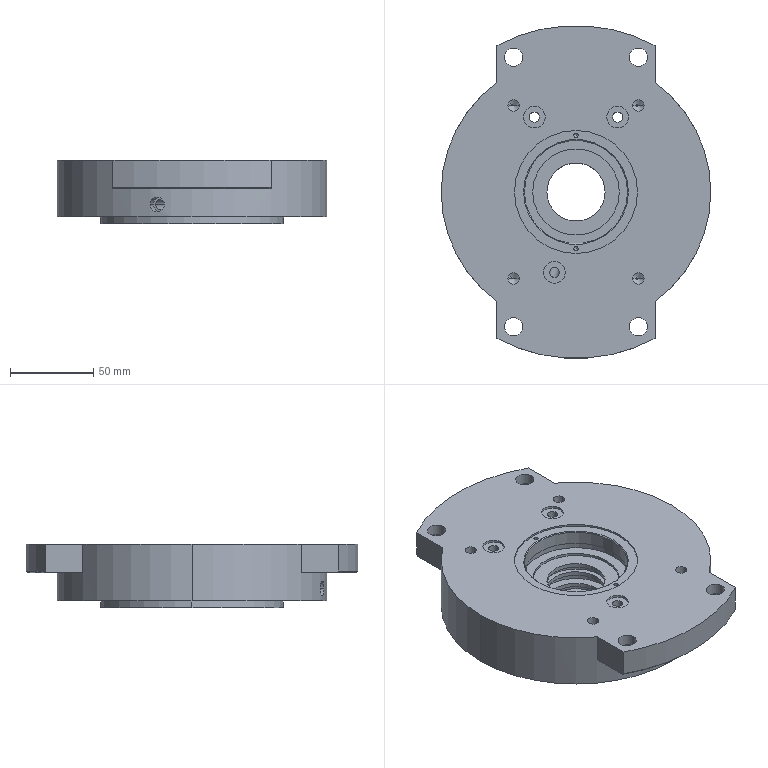Part | SolidWorks | features ICE 13, HoleWzd 9, Chamfer 2, 3DProfileFeature 1, CirPattern 1, Extrusion 1, MirrorPattern 1 | 1 solid | 157 faces | box 162 x 200 x 38 mm | volume 697983 mm3 | cylinder 94 | cone 36 | plane 27 | commonest cylinder face diameters 8.5 x16 6 x9 6.8 x8 11 x8 16 x8 35 x8